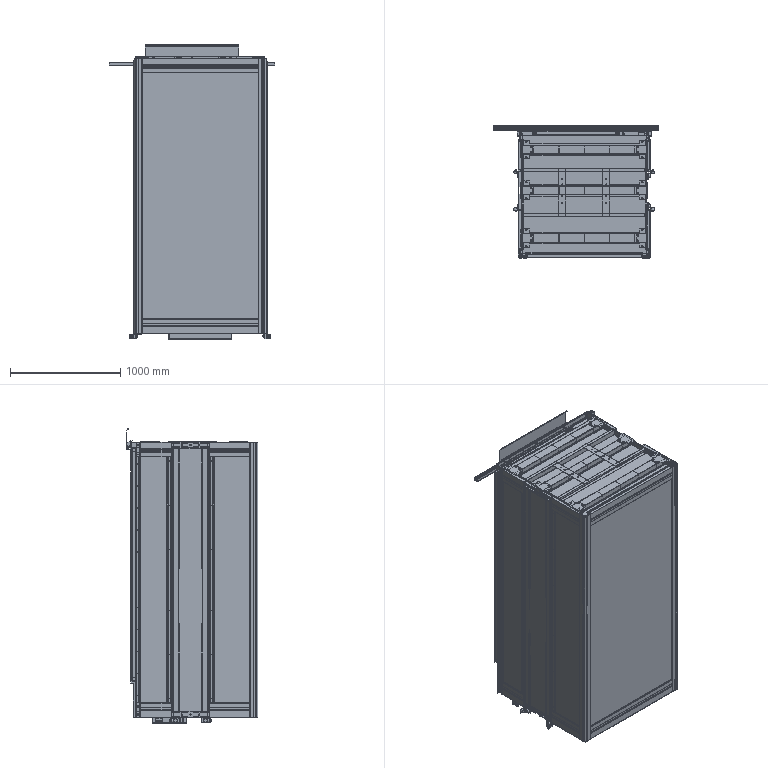Part | SolidWorks | features InContextFeatHolder 4 | 216 solids | 8075 faces | volume 120553237 mm3 | plane 5135 | cylinder 2566 | cone 336 | spline 38 | commonest cylinder face diameters 10 x256 0.4 x178 5 x160 6 x145 10.5 x134 6.2 x132